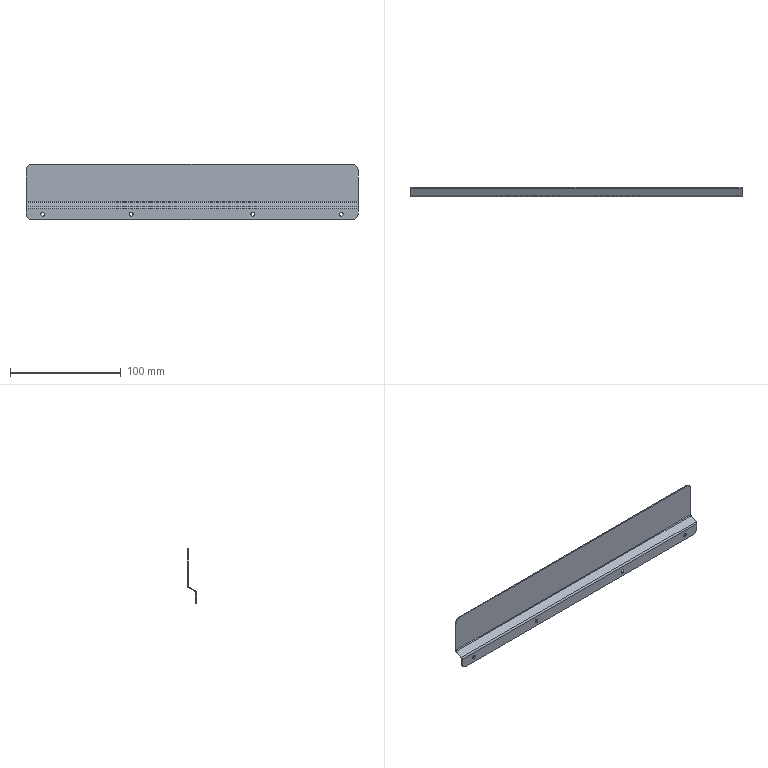Part | SolidWorks | features BaseBody 1 | 1 solid | 26 faces | box 300 x 8.861 x 50.116 mm | volume 16240 mm3 | cylinder 16 | plane 10 | commonest cylinder face diameters 3.5 x8 10 x4 2 x2 4 x2
STEP:
#1=CARTESIAN_POINT('',(-55.,-1.,-1.75));
#2=VERTEX_POINT('',#1);
#3=CARTESIAN_POINT('',(-55.,-1.,1.75));
#4=VERTEX_POINT('',#3);
#5=CARTESIAN_POINT('',(-55.,-1.,0.));
#6=DIRECTION('',(0.,1.,0.));
#7=DIRECTION('',(0.,0.,1.));
#8=AXIS2_PLACEMENT_3D('',#5,#6,#7);
#9=CIRCLE('',#8,1.75);
#10=EDGE_CURVE('',#2,#4,#9,.T.);
#11=ORIENTED_EDGE('',*,*,#10,.F.);
#12=CARTESIAN_POINT('',(-55.,0.,-1.75));
#13=VERTEX_POINT('',#12);
#14=CARTESIAN_POINT('',(-55.,7.861,-1.75));
#15=DIRECTION('',(0.,1.,0.));
#16=VECTOR('',#15,1000.);
#17=LINE('',#14,#16);
#18=EDGE_CURVE('',#2,#13,#17,.T.);
#19=ORIENTED_EDGE('',*,*,#18,.T.);
#20=CARTESIAN_POINT('',(-55.,0.,1.75));
#21=VERTEX_POINT('',#20);
#22=CARTESIAN_POINT('',(-55.,0.,0.));
#23=DIRECTION('',(0.,1.,0.));
#24=DIRECTION('',(0.,0.,1.));
#25=AXIS2_PLACEMENT_3D('',#22,#23,#24);
#26=CIRCLE('',#25,1.75);
#27=EDGE_CURVE('',#13,#21,#26,.T.);
#28=ORIENTED_EDGE('',*,*,#27,.T.);
#29=CARTESIAN_POINT('',(-55.,7.861,1.75));
#30=DIRECTION('',(0.,1.,0.));
#31=VECTOR('',#30,1000.);
#32=LINE('',#29,#31);
#33=EDGE_CURVE('',#4,#21,#32,.T.);
#34=ORIENTED_EDGE('',*,*,#33,.F.);
#35=EDGE_LOOP('',(#11,#19,#28,#34));
#36=FACE_OUTER_BOUND('',#35,.T.);
#37=CARTESIAN_POINT('',(-55.,7.861,0.));
#38=DIRECTION('',(0.,1.,0.));
#39=DIRECTION('',(0.,0.,1.));
#40=AXIS2_PLACEMENT_3D('',#37,#38,#39);
#41=CYLINDRICAL_SURFACE('',#40,1.75);
#42=ADVANCED_FACE('',(#36),#41,.F.);
#43=CARTESIAN_POINT('',(55.,-1.,-1.75));
#44=VERTEX_POINT('',#43);
#45=CARTESIAN_POINT('',(55.,-1.,1.75));
#46=VERTEX_POINT('',#45);
#47=CARTESIAN_POINT('',(55.,-1.,0.));
#48=DIRECTION('',(0.,1.,0.));
#49=DIRECTION('',(0.,0.,1.));
#50=AXIS2_PLACEMENT_3D('',#47,#48,#49);
#51=CIRCLE('',#50,1.75);
#52=EDGE_CURVE('',#44,#46,#51,.T.);
#53=ORIENTED_EDGE('',*,*,#52,.F.);
#54=CARTESIAN_POINT('',(55.,0.,-1.75));
#55=VERTEX_POINT('',#54);
#56=CARTESIAN_POINT('',(55.,7.861,-1.75));
#57=DIRECTION('',(0.,1.,0.));
#58=VECTOR('',#57,1000.);
#59=LINE('',#56,#58);
#60=EDGE_CURVE('',#44,#55,#59,.T.);
#61=ORIENTED_EDGE('',*,*,#60,.T.);
#62=CARTESIAN_POINT('',(55.,0.,1.75));
#63=VERTEX_POINT('',#62);
#64=CARTESIAN_POINT('',(55.,0.,0.));
#65=DIRECTION('',(0.,1.,0.));
#66=DIRECTION('',(0.,0.,1.));
#67=AXIS2_PLACEMENT_3D('',#64,#65,#66);
#68=CIRCLE('',#67,1.75);
#69=EDGE_CURVE('',#55,#63,#68,.T.);
#70=ORIENTED_EDGE('',*,*,#69,.T.);
#71=CARTESIAN_POINT('',(55.,7.861,1.75));
#72=DIRECTION('',(0.,1.,0.));
#73=VECTOR('',#72,1000.);
#74=LINE('',#71,#73);
#75=EDGE_CURVE('',#46,#63,#74,.T.);
#76=ORIENTED_EDGE('',*,*,#75,.F.);
#77=EDGE_LOOP('',(#53,#61,#70,#76));
#78=FACE_OUTER_BOUND('',#77,.T.);
#79=CARTESIAN_POINT('',(55.,7.861,0.));
#80=DIRECTION('',(0.,1.,0.));
#81=DIRECTION('',(0.,0.,1.));
#82=AXIS2_PLACEMENT_3D('',#79,#80,#81);
#83=CYLINDRICAL_SURFACE('',#82,1.75);
#84=ADVANCED_FACE('',(#78),#83,.F.);
#85=CARTESIAN_POINT('',(135.,-1.,-1.75));
#86=VERTEX_POINT('',#85);
#87=CARTESIAN_POINT('',(135.,-1.,1.75));
#88=VERTEX_POINT('',#87);
#89=CARTESIAN_POINT('',(135.,-1.,0.));
#90=DIRECTION('',(0.,1.,0.));
#91=DIRECTION('',(0.,0.,1.));
#92=AXIS2_PLACEMENT_3D('',#89,#90,#91);
#93=CIRCLE('',#92,1.75);
#94=EDGE_CURVE('',#86,#88,#93,.T.);
#95=ORIENTED_EDGE('',*,*,#94,.F.);
#96=CARTESIAN_POINT('',(135.,0.,-1.75));
#97=VERTEX_POINT('',#96);
#98=CARTESIAN_POINT('',(135.,7.861,-1.75));
#99=DIRECTION('',(0.,1.,0.));
#100=VECTOR('',#99,1000.);
#101=LINE('',#98,#100);
#102=EDGE_CURVE('',#86,#97,#101,.T.);
#103=ORIENTED_EDGE('',*,*,#102,.T.);
#104=CARTESIAN_POINT('',(135.,0.,1.75));
#105=VERTEX_POINT('',#104);
#106=CARTESIAN_POINT('',(135.,0.,0.));
#107=DIRECTION('',(0.,1.,0.));
#108=DIRECTION('',(0.,0.,1.));
#109=AXIS2_PLACEMENT_3D('',#106,#107,#108);
#110=CIRCLE('',#109,1.75);
#111=EDGE_CURVE('',#97,#105,#110,.T.);
#112=ORIENTED_EDGE('',*,*,#111,.T.);
#113=CARTESIAN_POINT('',(135.,7.861,1.75));
#114=DIRECTION('',(0.,1.,0.));
#115=VECTOR('',#114,1000.);
#116=LINE('',#113,#115);
#117=EDGE_CURVE('',#88,#105,#116,.T.);
#118=ORIENTED_EDGE('',*,*,#117,.F.);
#119=EDGE_LOOP('',(#95,#103,#112,#118));
#120=FACE_OUTER_BOUND('',#119,.T.);
#121=CARTESIAN_POINT('',(135.,7.861,0.));
#122=DIRECTION('',(0.,1.,0.));
#123=DIRECTION('',(0.,0.,1.));
#124=AXIS2_PLACEMENT_3D('',#121,#122,#123);
#125=CYLINDRICAL_SURFACE('',#124,1.75);
#126=ADVANCED_FACE('',(#120),#125,.F.);
#127=CARTESIAN_POINT('',(-135.,-1.,-1.75));
#128=VERTEX_POINT('',#127);
#129=CARTESIAN_POINT('',(-135.,-1.,1.75));
#130=VERTEX_POINT('',#129);
#131=CARTESIAN_POINT('',(-135.,-1.,0.));
#132=DIRECTION('',(0.,1.,0.));
#133=DIRECTION('',(0.,0.,1.));
#134=AXIS2_PLACEMENT_3D('',#131,#132,#133);
#135=CIRCLE('',#134,1.75);
#136=EDGE_CURVE('',#128,#130,#135,.T.);
#137=ORIENTED_EDGE('',*,*,#136,.F.);
#138=CARTESIAN_POINT('',(-135.,0.,-1.75));
#139=VERTEX_POINT('',#138);
#140=CARTESIAN_POINT('',(-135.,7.861,-1.75));
#141=DIRECTION('',(0.,1.,0.));
#142=VECTOR('',#141,1000.);
#143=LINE('',#140,#142);
#144=EDGE_CURVE('',#128,#139,#143,.T.);
#145=ORIENTED_EDGE('',*,*,#144,.T.);
#146=CARTESIAN_POINT('',(-135.,0.,1.75));
#147=VERTEX_POINT('',#146);
#148=CARTESIAN_POINT('',(-135.,0.,0.));
#149=DIRECTION('',(0.,1.,0.));
#150=DIRECTION('',(0.,0.,1.));
#151=AXIS2_PLACEMENT_3D('',#148,#149,#150);
#152=CIRCLE('',#151,1.75);
#153=EDGE_CURVE('',#139,#147,#152,.T.);
#154=ORIENTED_EDGE('',*,*,#153,.T.);
#155=CARTESIAN_POINT('',(-135.,7.861,1.75));
#156=DIRECTION('',(0.,1.,0.));
#157=VECTOR('',#156,1000.);
#158=LINE('',#155,#157);
#159=EDGE_CURVE('',#130,#147,#158,.T.);
#160=ORIENTED_EDGE('',*,*,#159,.F.);
#161=EDGE_LOOP('',(#137,#145,#154,#160));
#162=FACE_OUTER_BOUND('',#161,.T.);
#163=CARTESIAN_POINT('',(-135.,7.861,0.));
#164=DIRECTION('',(0.,1.,0.));
#165=DIRECTION('',(0.,0.,1.));
#166=AXIS2_PLACEMENT_3D('',#163,#164,#165);
#167=CYLINDRICAL_SURFACE('',#166,1.75);
#168=ADVANCED_FACE('',(#162),#167,.F.);
#169=CARTESIAN_POINT('',(-150.,7.861,40.116));
#170=VERTEX_POINT('',#169);
#171=CARTESIAN_POINT('',(-145.,7.861,45.116));
#172=VERTEX_POINT('',#171);
#173=CARTESIAN_POINT('',(-145.,7.861,40.116));
#174=DIRECTION('',(0.,1.,0.));
#175=DIRECTION('',(0.,0.,-1.));
#176=AXIS2_PLACEMENT_3D('',#173,#174,#175);
#177=CIRCLE('',#176,5.);
#178=EDGE_CURVE('',#170,#172,#177,.T.);
#179=ORIENTED_EDGE('',*,*,#178,.F.);
#180=CARTESIAN_POINT('',(-150.,6.861,40.116));
#181=VERTEX_POINT('',#180);
#182=CARTESIAN_POINT('',(-150.,7.861,40.116));
#183=DIRECTION('',(0.,1.,0.));
#184=VECTOR('',#183,1000.);
#185=LINE('',#182,#184);
#186=EDGE_CURVE('',#181,#170,#185,.T.);
#187=ORIENTED_EDGE('',*,*,#186,.F.);
#188=CARTESIAN_POINT('',(-145.,6.861,45.116));
#189=VERTEX_POINT('',#188);
#190=CARTESIAN_POINT('',(-145.,6.861,40.116));
#191=DIRECTION('',(0.,-1.,0.));
#192=DIRECTION('',(0.,0.,-1.));
#193=AXIS2_PLACEMENT_3D('',#190,#191,#192);
#194=CIRCLE('',#193,5.);
#195=EDGE_CURVE('',#189,#181,#194,.T.);
#196=ORIENTED_EDGE('',*,*,#195,.F.);
#197=CARTESIAN_POINT('',(-145.,7.861,45.116));
#198=DIRECTION('',(0.,-1.,0.));
#199=VECTOR('',#198,1000.);
#200=LINE('',#197,#199);
#201=EDGE_CURVE('',#172,#189,#200,.T.);
#202=ORIENTED_EDGE('',*,*,#201,.F.);
#203=EDGE_LOOP('',(#179,#187,#196,#202));
#204=FACE_OUTER_BOUND('',#203,.T.);
#205=CARTESIAN_POINT('',(-145.,7.861,40.116));
#206=DIRECTION('',(0.,-1.,0.));
#207=DIRECTION('',(0.,0.,-1.));
#208=AXIS2_PLACEMENT_3D('',#205,#206,#207);
#209=CYLINDRICAL_SURFACE('',#208,5.);
#210=ADVANCED_FACE('',(#204),#209,.T.);
#211=CARTESIAN_POINT('',(145.,7.861,45.116));
#212=VERTEX_POINT('',#211);
#213=CARTESIAN_POINT('',(150.,7.861,40.116));
#214=VERTEX_POINT('',#213);
#215=CARTESIAN_POINT('',(145.,7.861,40.116));
#216=DIRECTION('',(0.,1.,0.));
#217=DIRECTION('',(0.,0.,-1.));
#218=AXIS2_PLACEMENT_3D('',#215,#216,#217);
#219=CIRCLE('',#218,5.);
#220=EDGE_CURVE('',#212,#214,#219,.T.);
#221=ORIENTED_EDGE('',*,*,#220,.F.);
#222=CARTESIAN_POINT('',(145.,6.861,45.116));
#223=VERTEX_POINT('',#222);
#224=CARTESIAN_POINT('',(145.,7.861,45.116));
#225=DIRECTION('',(0.,1.,0.));
#226=VECTOR('',#225,1000.);
#227=LINE('',#224,#226);
#228=EDGE_CURVE('',#223,#212,#227,.T.);
#229=ORIENTED_EDGE('',*,*,#228,.F.);
#230=CARTESIAN_POINT('',(150.,6.861,40.116));
#231=VERTEX_POINT('',#230);
#232=CARTESIAN_POINT('',(145.,6.861,40.116));
#233=DIRECTION('',(0.,-1.,0.));
#234=DIRECTION('',(0.,0.,-1.));
#235=AXIS2_PLACEMENT_3D('',#232,#233,#234);
#236=CIRCLE('',#235,5.);
#237=EDGE_CURVE('',#231,#223,#236,.T.);
#238=ORIENTED_EDGE('',*,*,#237,.F.);
#239=CARTESIAN_POINT('',(150.,7.861,40.116));
#240=DIRECTION('',(0.,-1.,0.));
#241=VECTOR('',#240,1000.);
#242=LINE('',#239,#241);
#243=EDGE_CURVE('',#214,#231,#242,.T.);
#244=ORIENTED_EDGE('',*,*,#243,.F.);
#245=EDGE_LOOP('',(#221,#229,#238,#244));
#246=FACE_OUTER_BOUND('',#245,.T.);
#247=CARTESIAN_POINT('',(145.,7.861,40.116));
#248=DIRECTION('',(0.,-1.,0.));
#249=DIRECTION('',(0.,0.,-1.));
#250=AXIS2_PLACEMENT_3D('',#247,#248,#249);
#251=CYLINDRICAL_SURFACE('',#250,5.);
#252=ADVANCED_FACE('',(#246),#251,.T.);
#253=CARTESIAN_POINT('',(-150.,-1.,0.));
#254=VERTEX_POINT('',#253);
#255=CARTESIAN_POINT('',(-145.,-1.,-5.));
#256=VERTEX_POINT('',#255);
#257=CARTESIAN_POINT('',(-145.,-1.,0.));
#258=DIRECTION('',(0.,-1.,0.));
#259=DIRECTION('',(0.,0.,1.));
#260=AXIS2_PLACEMENT_3D('',#257,#258,#259);
#261=CIRCLE('',#260,5.);
#262=EDGE_CURVE('',#254,#256,#261,.T.);
#263=ORIENTED_EDGE('',*,*,#262,.F.);
#264=CARTESIAN_POINT('',(-150.,0.,0.));
#265=VERTEX_POINT('',#264);
#266=CARTESIAN_POINT('',(-150.,-1.,0.));
#267=DIRECTION('',(0.,-1.,0.));
#268=VECTOR('',#267,1000.);
#269=LINE('',#266,#268);
#270=EDGE_CURVE('',#265,#254,#269,.T.);
#271=ORIENTED_EDGE('',*,*,#270,.F.);
#272=CARTESIAN_POINT('',(-145.,0.,-5.));
#273=VERTEX_POINT('',#272);
#274=CARTESIAN_POINT('',(-145.,0.,0.));
#275=DIRECTION('',(0.,1.,0.));
#276=DIRECTION('',(0.,0.,1.));
#277=AXIS2_PLACEMENT_3D('',#274,#275,#276);
#278=CIRCLE('',#277,5.);
#279=EDGE_CURVE('',#273,#265,#278,.T.);
#280=ORIENTED_EDGE('',*,*,#279,.F.);
#281=CARTESIAN_POINT('',(-145.,-1.,-5.));
#282=DIRECTION('',(0.,1.,0.));
#283=VECTOR('',#282,1000.);
#284=LINE('',#281,#283);
#285=EDGE_CURVE('',#256,#273,#284,.T.);
#286=ORIENTED_EDGE('',*,*,#285,.F.);
#287=EDGE_LOOP('',(#263,#271,#280,#286));
#288=FACE_OUTER_BOUND('',#287,.T.);
#289=CARTESIAN_POINT('',(-145.,-1.,0.));
#290=DIRECTION('',(0.,1.,0.));
#291=DIRECTION('',(0.,0.,1.));
#292=AXIS2_PLACEMENT_3D('',#289,#290,#291);
#293=CYLINDRICAL_SURFACE('',#292,5.);
#294=ADVANCED_FACE('',(#288),#293,.T.);
#295=CARTESIAN_POINT('',(145.,-1.,-5.));
#296=VERTEX_POINT('',#295);
#297=CARTESIAN_POINT('',(150.,-1.,0.));
#298=VERTEX_POINT('',#297);
#299=CARTESIAN_POINT('',(145.,-1.,0.));
#300=DIRECTION('',(0.,-1.,0.));
#301=DIRECTION('',(0.,0.,1.));
#302=AXIS2_PLACEMENT_3D('',#299,#300,#301);
#303=CIRCLE('',#302,5.);
#304=EDGE_CURVE('',#296,#298,#303,.T.);
#305=ORIENTED_EDGE('',*,*,#304,.F.);
#306=CARTESIAN_POINT('',(145.,0.,-5.));
#307=VERTEX_POINT('',#306);
#308=CARTESIAN_POINT('',(145.,-1.,-5.));
#309=DIRECTION('',(0.,-1.,0.));
#310=VECTOR('',#309,1000.);
#311=LINE('',#308,#310);
#312=EDGE_CURVE('',#307,#296,#311,.T.);
#313=ORIENTED_EDGE('',*,*,#312,.F.);
#314=CARTESIAN_POINT('',(150.,0.,0.));
#315=VERTEX_POINT('',#314);
#316=CARTESIAN_POINT('',(145.,0.,0.));
#317=DIRECTION('',(0.,1.,0.));
#318=DIRECTION('',(0.,0.,1.));
#319=AXIS2_PLACEMENT_3D('',#316,#317,#318);
#320=CIRCLE('',#319,5.);
#321=EDGE_CURVE('',#315,#307,#320,.T.);
#322=ORIENTED_EDGE('',*,*,#321,.F.);
#323=CARTESIAN_POINT('',(150.,-1.,0.));
#324=DIRECTION('',(0.,1.,0.));
#325=VECTOR('',#324,1000.);
#326=LINE('',#323,#325);
#327=EDGE_CURVE('',#298,#315,#326,.T.);
#328=ORIENTED_EDGE('',*,*,#327,.F.);
#329=EDGE_LOOP('',(#305,#313,#322,#328));
#330=FACE_OUTER_BOUND('',#329,.T.);
#331=CARTESIAN_POINT('',(145.,-1.,0.));
#332=DIRECTION('',(0.,1.,0.));
#333=DIRECTION('',(0.,0.,1.));
#334=AXIS2_PLACEMENT_3D('',#331,#332,#333);
#335=CYLINDRICAL_SURFACE('',#334,5.);
#336=ADVANCED_FACE('',(#330),#335,.T.);
#337=CARTESIAN_POINT('',(150.,6.861,45.116));
#338=DIRECTION('',(1.,0.,0.));
#339=VECTOR('',#338,1000.);
#340=LINE('',#337,#339);
#341=EDGE_CURVE('',#189,#223,#340,.T.);
#342=ORIENTED_EDGE('',*,*,#341,.T.);
#343=ORIENTED_EDGE('',*,*,#228,.T.);
#344=CARTESIAN_POINT('',(0.,7.861,45.116));
#345=DIRECTION('',(1.,0.,0.));
#346=VECTOR('',#345,1000.);
#347=LINE('',#344,#346);
#348=EDGE_CURVE('',#172,#212,#347,.T.);
#349=ORIENTED_EDGE('',*,*,#348,.F.);
#350=ORIENTED_EDGE('',*,*,#201,.T.);
#351=EDGE_LOOP('',(#342,#343,#349,#350));
#352=FACE_OUTER_BOUND('',#351,.T.);
#353=CARTESIAN_POINT('',(150.,7.861,45.116));
#354=DIRECTION('',(0.,0.,-1.));
#355=DIRECTION('',(-1.,0.,0.));
#356=AXIS2_PLACEMENT_3D('',#353,#354,#355);
#357=PLANE('',#356);
#358=ADVANCED_FACE('',(#352),#357,.F.);
#359=CARTESIAN_POINT('',(150.,6.861,11.271));
#360=VERTEX_POINT('',#359);
#361=CARTESIAN_POINT('',(150.,6.861,10.693));
#362=DIRECTION('',(0.,0.,-1.));
#363=VECTOR('',#362,1000.);
#364=LINE('',#361,#363);
#365=EDGE_CURVE('',#231,#360,#364,.T.);
#366=ORIENTED_EDGE('',*,*,#365,.F.);
#367=ORIENTED_EDGE('',*,*,#237,.T.);
#368=ORIENTED_EDGE('',*,*,#341,.F.);
#369=ORIENTED_EDGE('',*,*,#195,.T.);
#370=CARTESIAN_POINT('',(-150.,6.861,11.271));
#371=VERTEX_POINT('',#370);
#372=CARTESIAN_POINT('',(-150.,6.861,45.116));
#373=DIRECTION('',(0.,0.,1.));
#374=VECTOR('',#373,1000.);
#375=LINE('',#372,#374);
#376=EDGE_CURVE('',#371,#181,#375,.T.);
#377=ORIENTED_EDGE('',*,*,#376,.F.);
#378=CARTESIAN_POINT('',(150.,6.861,11.271));
#379=DIRECTION('',(-1.,0.,0.));
#380=VECTOR('',#379,1000.);
#381=LINE('',#378,#380);
#382=EDGE_CURVE('',#360,#371,#381,.T.);
#383=ORIENTED_EDGE('',*,*,#382,.F.);
#384=EDGE_LOOP('',(#366,#367,#368,#369,#377,#383));
#385=FACE_OUTER_BOUND('',#384,.T.);
#386=CARTESIAN_POINT('',(0.,6.861,0.2887));
#387=DIRECTION('',(0.,-1.,0.));
#388=DIRECTION('',(0.,0.,-1.));
#389=AXIS2_PLACEMENT_3D('',#386,#387,#388);
#390=PLANE('',#389);
#391=ADVANCED_FACE('',(#385),#390,.T.);
#392=ORIENTED_EDGE('',*,*,#348,.T.);
#393=ORIENTED_EDGE('',*,*,#220,.T.);
#394=CARTESIAN_POINT('',(150.,7.861,11.271));
#395=VERTEX_POINT('',#394);
#396=CARTESIAN_POINT('',(150.,7.861,0.2887));
#397=DIRECTION('',(0.,0.,-1.));
#398=VECTOR('',#397,1000.);
#399=LINE('',#396,#398);
#400=EDGE_CURVE('',#214,#395,#399,.T.);
#401=ORIENTED_EDGE('',*,*,#400,.T.);
#402=CARTESIAN_POINT('',(-150.,7.861,11.271));
#403=VERTEX_POINT('',#402);
#404=CARTESIAN_POINT('',(150.,7.861,11.271));
#405=DIRECTION('',(1.,0.,0.));
#406=VECTOR('',#405,1000.);
#407=LINE('',#404,#406);
#408=EDGE_CURVE('',#403,#395,#407,.T.);
#409=ORIENTED_EDGE('',*,*,#408,.F.);
#410=CARTESIAN_POINT('',(-150.,7.861,0.2887));
#411=DIRECTION('',(0.,0.,1.));
#412=VECTOR('',#411,1000.);
#413=LINE('',#410,#412);
#414=EDGE_CURVE('',#403,#170,#413,.T.);
#415=ORIENTED_EDGE('',*,*,#414,.T.);
#416=ORIENTED_EDGE('',*,*,#178,.T.);
#417=EDGE_LOOP('',(#392,#393,#401,#409,#415,#416));
#418=FACE_OUTER_BOUND('',#417,.T.);
#419=CARTESIAN_POINT('',(0.,7.861,0.2887));
#420=DIRECTION('',(0.,-1.,0.));
#421=DIRECTION('',(0.,0.,-1.));
#422=AXIS2_PLACEMENT_3D('',#419,#420,#421);
#423=PLANE('',#422);
#424=ADVANCED_FACE('',(#418),#423,.F.);
#425=CARTESIAN_POINT('',(150.,6.361,10.405));
#426=VERTEX_POINT('',#425);
#427=CARTESIAN_POINT('',(-150.,6.361,10.405));
#428=VERTEX_POINT('',#427);
#429=CARTESIAN_POINT('',(0.,6.361,10.405));
#430=DIRECTION('',(-1.,0.,0.));
#431=VECTOR('',#430,1000.);
#432=LINE('',#429,#431);
#433=EDGE_CURVE('',#426,#428,#432,.T.);
#434=ORIENTED_EDGE('',*,*,#433,.F.);
#435=CARTESIAN_POINT('',(150.,5.861,11.271));
#436=DIRECTION('',(1.,0.,0.));
#437=DIRECTION('',(0.,0.,1.));
#438=AXIS2_PLACEMENT_3D('',#435,#436,#437);
#439=CIRCLE('',#438,1.);
#440=EDGE_CURVE('',#426,#360,#439,.T.);
#441=ORIENTED_EDGE('',*,*,#440,.T.);
#442=ORIENTED_EDGE('',*,*,#382,.T.);
#443=CARTESIAN_POINT('',(-150.,5.861,11.271));
#444=DIRECTION('',(-1.,0.,0.));
#445=DIRECTION('',(0.,0.,1.));
#446=AXIS2_PLACEMENT_3D('',#443,#444,#445);
#447=CIRCLE('',#446,1.);
#448=EDGE_CURVE('',#371,#428,#447,.T.);
#449=ORIENTED_EDGE('',*,*,#448,.T.);
#450=EDGE_LOOP('',(#434,#441,#442,#449));
#451=FACE_OUTER_BOUND('',#450,.T.);
#452=CARTESIAN_POINT('',(-150.,5.861,11.271));
#453=DIRECTION('',(-1.,0.,0.));
#454=DIRECTION('',(0.,1.,0.));
#455=AXIS2_PLACEMENT_3D('',#452,#453,#454);
#456=CYLINDRICAL_SURFACE('',#455,1.);
#457=ADVANCED_FACE('',(#451),#456,.F.);
#458=CARTESIAN_POINT('',(150.,6.861,9.539));
#459=VERTEX_POINT('',#458);
#460=CARTESIAN_POINT('',(-150.,6.861,9.539));
#461=VERTEX_POINT('',#460);
#462=CARTESIAN_POINT('',(-150.,6.861,9.539));
#463=DIRECTION('',(-1.,0.,0.));
#464=VECTOR('',#463,1000.);
#465=LINE('',#462,#464);
#466=EDGE_CURVE('',#459,#461,#465,.T.);
#467=ORIENTED_EDGE('',*,*,#466,.T.);
#468=CARTESIAN_POINT('',(-150.,5.861,11.271));
#469=DIRECTION('',(-1.,0.,0.));
#470=DIRECTION('',(0.,0.,1.));
#471=AXIS2_PLACEMENT_3D('',#468,#469,#470);
#472=CIRCLE('',#471,2.);
#473=EDGE_CURVE('',#403,#461,#472,.T.);
#474=ORIENTED_EDGE('',*,*,#473,.F.);
#475=ORIENTED_EDGE('',*,*,#408,.T.);
#476=CARTESIAN_POINT('',(150.,5.861,11.271));
#477=DIRECTION('',(1.,0.,0.));
#478=DIRECTION('',(0.,0.,1.));
#479=AXIS2_PLACEMENT_3D('',#476,#477,#478);
#480=CIRCLE('',#479,2.);
#481=EDGE_CURVE('',#459,#395,#480,.T.);
#482=ORIENTED_EDGE('',*,*,#481,.F.);
#483=EDGE_LOOP('',(#467,#474,#475,#482));
#484=FACE_OUTER_BOUND('',#483,.T.);
#485=CARTESIAN_POINT('',(-150.,5.861,11.271));
#486=DIRECTION('',(-1.,0.,0.));
#487=DIRECTION('',(0.,1.,0.));
#488=AXIS2_PLACEMENT_3D('',#485,#486,#487);
#489=CYLINDRICAL_SURFACE('',#488,2.);
#490=ADVANCED_FACE('',(#484),#489,.T.);
#491=CARTESIAN_POINT('',(150.,0.5,5.866));
#492=VERTEX_POINT('',#491);
#493=CARTESIAN_POINT('',(150.,6.861,9.539));
#494=DIRECTION('',(0.,0.866,0.5));
#495=VECTOR('',#494,1000.);
#496=LINE('',#493,#495);
#497=EDGE_CURVE('',#492,#459,#496,.T.);
#498=ORIENTED_EDGE('',*,*,#497,.F.);
#499=CARTESIAN_POINT('',(-150.,0.5,5.866));
#500=VERTEX_POINT('',#499);
#501=CARTESIAN_POINT('',(-150.,0.5,5.866));
#502=DIRECTION('',(1.,0.,0.));
#503=VECTOR('',#502,1000.);
#504=LINE('',#501,#503);
#505=EDGE_CURVE('',#500,#492,#504,.T.);
#506=ORIENTED_EDGE('',*,*,#505,.F.);
#507=CARTESIAN_POINT('',(-150.,0.,5.577));
#508=DIRECTION('',(0.,-0.866,-0.5));
#509=VECTOR('',#508,1000.);
#510=LINE('',#507,#509);
#511=EDGE_CURVE('',#461,#500,#510,.T.);
#512=ORIENTED_EDGE('',*,*,#511,.F.);
#513=ORIENTED_EDGE('',*,*,#466,.F.);
#514=EDGE_LOOP('',(#498,#506,#512,#513));
#515=FACE_OUTER_BOUND('',#514,.T.);
#516=CARTESIAN_POINT('',(0.,-2.165,4.327));
#517=DIRECTION('',(0.,0.5,-0.866));
#518=DIRECTION('',(-1.,0.,0.));
#519=AXIS2_PLACEMENT_3D('',#516,#517,#518);
#520=PLANE('',#519);
#521=ADVANCED_FACE('',(#515),#520,.T.);
#522=CARTESIAN_POINT('',(150.,0.,6.732));
#523=VERTEX_POINT('',#522);
#524=CARTESIAN_POINT('',(-150.,0.,6.732));
#525=VERTEX_POINT('',#524);
#526=CARTESIAN_POINT('',(-150.,0.,6.732));
#527=DIRECTION('',(-1.,0.,0.));
#528=VECTOR('',#527,1000.);
#529=LINE('',#526,#528);
#530=EDGE_CURVE('',#523,#525,#529,.T.);
#531=ORIENTED_EDGE('',*,*,#530,.F.);
#532=CARTESIAN_POINT('',(150.,-2.665,5.193));
#533=DIRECTION('',(0.,0.866,0.5));
#534=VECTOR('',#533,1000.);
#535=LINE('',#532,#534);
#536=EDGE_CURVE('',#523,#426,#535,.T.);
#537=ORIENTED_EDGE('',*,*,#536,.T.);
#538=ORIENTED_EDGE('',*,*,#433,.T.);
#539=CARTESIAN_POINT('',(-150.,-2.665,5.193));
#540=DIRECTION('',(0.,-0.866,-0.5));
#541=VECTOR('',#540,1000.);
#542=LINE('',#539,#541);
#543=EDGE_CURVE('',#428,#525,#542,.T.);
#544=ORIENTED_EDGE('',*,*,#543,.T.);
#545=EDGE_LOOP('',(#531,#537,#538,#544));
#546=FACE_OUTER_BOUND('',#545,.T.);
#547=CARTESIAN_POINT('',(0.,-2.665,5.193));
#548=DIRECTION('',(0.,0.5,-0.866));
#549=DIRECTION('',(-1.,0.,0.));
#550=AXIS2_PLACEMENT_3D('',#547,#548,#549);
#551=PLANE('',#550);
#552=ADVANCED_FACE('',(#546),#551,.F.);
#553=CARTESIAN_POINT('',(-150.,0.,5.));
#554=VERTEX_POINT('',#553);
#555=CARTESIAN_POINT('',(150.,0.,5.));
#556=VERTEX_POINT('',#555);
#557=CARTESIAN_POINT('',(-150.,0.,5.));
#558=DIRECTION('',(1.,0.,0.));
#559=VECTOR('',#558,1000.);
#560=LINE('',#557,#559);
#561=EDGE_CURVE('',#554,#556,#560,.T.);
#562=ORIENTED_EDGE('',*,*,#561,.F.);
#563=CARTESIAN_POINT('',(-150.,1.,5.));
#564=DIRECTION('',(-1.,0.,0.));
#565=DIRECTION('',(0.,0.,-1.));
#566=AXIS2_PLACEMENT_3D('',#563,#564,#565);
#567=CIRCLE('',#566,1.);
#568=EDGE_CURVE('',#554,#500,#567,.T.);
#569=ORIENTED_EDGE('',*,*,#568,.T.);
#570=ORIENTED_EDGE('',*,*,#505,.T.);
#571=CARTESIAN_POINT('',(150.,1.,5.));
#572=DIRECTION('',(1.,0.,0.));
#573=DIRECTION('',(0.,0.,-1.));
#574=AXIS2_PLACEMENT_3D('',#571,#572,#573);
#575=CIRCLE('',#574,1.);
#576=EDGE_CURVE('',#492,#556,#575,.T.);
#577=ORIENTED_EDGE('',*,*,#576,.T.);
#578=EDGE_LOOP('',(#562,#569,#570,#577));
#579=FACE_OUTER_BOUND('',#578,.T.);
#580=CARTESIAN_POINT('',(150.,1.,5.));
#581=DIRECTION('',(1.,0.,0.));
#582=DIRECTION('',(0.,-0.5,0.866));
#583=AXIS2_PLACEMENT_3D('',#580,#581,#582);
#584=CYLINDRICAL_SURFACE('',#583,1.);
#585=ADVANCED_FACE('',(#579),#584,.F.);
#586=CARTESIAN_POINT('',(-150.,-1.,5.));
#587=VERTEX_POINT('',#586);
#588=CARTESIAN_POINT('',(150.,-1.,5.));
#589=VERTEX_POINT('',#588);
#590=CARTESIAN_POINT('',(-150.,-1.,5.));
#591=DIRECTION('',(1.,0.,0.));
#592=VECTOR('',#591,1000.);
#593=LINE('',#590,#592);
#594=EDGE_CURVE('',#587,#589,#593,.T.);
#595=ORIENTED_EDGE('',*,*,#594,.T.);
#596=CARTESIAN_POINT('',(150.,1.,5.));
#597=DIRECTION('',(1.,0.,0.));
#598=DIRECTION('',(0.,0.,-1.));
#599=AXIS2_PLACEMENT_3D('',#596,#597,#598);
#600=CIRCLE('',#599,2.);
#601=EDGE_CURVE('',#523,#589,#600,.T.);
#602=ORIENTED_EDGE('',*,*,#601,.F.);
#603=ORIENTED_EDGE('',*,*,#530,.T.);
#604=CARTESIAN_POINT('',(-150.,1.,5.));
#605=DIRECTION('',(-1.,0.,0.));
#606=DIRECTION('',(0.,0.,-1.));
#607=AXIS2_PLACEMENT_3D('',#604,#605,#606);
#608=CIRCLE('',#607,2.);
#609=EDGE_CURVE('',#587,#525,#608,.T.);
#610=ORIENTED_EDGE('',*,*,#609,.F.);
#611=EDGE_LOOP('',(#595,#602,#603,#610));
#612=FACE_OUTER_BOUND('',#611,.T.);
#613=CARTESIAN_POINT('',(150.,1.,5.));
#614=DIRECTION('',(1.,0.,0.));
#615=DIRECTION('',(0.,-0.5,0.866));
#616=AXIS2_PLACEMENT_3D('',#613,#614,#615);
#617=CYLINDRICAL_SURFACE('',#616,2.);
#618=ADVANCED_FACE('',(#612),#617,.T.);
#619=CARTESIAN_POINT('',(-135.,0.,0.));
#620=DIRECTION('',(0.,1.,0.));
#621=DIRECTION('',(0.,0.,1.));
#622=AXIS2_PLACEMENT_3D('',#619,#620,#621);
#623=CIRCLE('',#622,1.75);
#624=EDGE_CURVE('',#147,#139,#623,.T.);
#625=ORIENTED_EDGE('',*,*,#624,.F.);
#626=ORIENTED_EDGE('',*,*,#153,.F.);
#627=EDGE_LOOP('',(#625,#626));
#628=FACE_BOUND('',#627,.T.);
#629=CARTESIAN_POINT('',(135.,0.,0.));
#630=DIRECTION('',(0.,1.,0.));
#631=DIRECTION('',(0.,0.,1.));
#632=AXIS2_PLACEMENT_3D('',#629,#630,#631);
#633=CIRCLE('',#632,1.75);
#634=EDGE_CURVE('',#105,#97,#633,.T.);
#635=ORIENTED_EDGE('',*,*,#634,.F.);
#636=ORIENTED_EDGE('',*,*,#111,.F.);
#637=EDGE_LOOP('',(#635,#636));
#638=FACE_BOUND('',#637,.T.);
#639=CARTESIAN_POINT('',(55.,0.,0.));
#640=DIRECTION('',(0.,1.,0.));
#641=DIRECTION('',(0.,0.,1.));
#642=AXIS2_PLACEMENT_3D('',#639,#640,#641);
#643=CIRCLE('',#642,1.75);
#644=EDGE_CURVE('',#63,#55,#643,.T.);
#645=ORIENTED_EDGE('',*,*,#644,.F.);
#646=ORIENTED_EDGE('',*,*,#69,.F.);
#647=EDGE_LOOP('',(#645,#646));
#648=FACE_BOUND('',#647,.T.);
#649=CARTESIAN_POINT('',(-55.,0.,0.));
#650=DIRECTION('',(0.,1.,0.));
#651=DIRECTION('',(0.,0.,1.));
#652=AXIS2_PLACEMENT_3D('',#649,#650,#651);
#653=CIRCLE('',#652,1.75);
#654=EDGE_CURVE('',#21,#13,#653,.T.);
#655=ORIENTED_EDGE('',*,*,#654,.F.);
#656=ORIENTED_EDGE('',*,*,#27,.F.);
#657=EDGE_LOOP('',(#655,#656));
#658=FACE_BOUND('',#657,.T.);
#659=CARTESIAN_POINT('',(150.,0.,-5.));
#660=DIRECTION('',(0.,0.,-1.));
#661=VECTOR('',#660,1000.);
#662=LINE('',#659,#661);
#663=EDGE_CURVE('',#556,#315,#662,.T.);
#664=ORIENTED_EDGE('',*,*,#663,.T.);
#665=ORIENTED_EDGE('',*,*,#321,.T.);
#666=CARTESIAN_POINT('',(-150.,0.,-5.));
#667=DIRECTION('',(-1.,0.,0.));
#668=VECTOR('',#667,1000.);
#669=LINE('',#666,#668);
#670=EDGE_CURVE('',#307,#273,#669,.T.);
#671=ORIENTED_EDGE('',*,*,#670,.T.);
#672=ORIENTED_EDGE('',*,*,#279,.T.);
#673=CARTESIAN_POINT('',(-150.,0.,-5.));
#674=DIRECTION('',(0.,0.,1.));
#675=VECTOR('',#674,1000.);
#676=LINE('',#673,#675);
#677=EDGE_CURVE('',#265,#554,#676,.T.);
#678=ORIENTED_EDGE('',*,*,#677,.T.);
#679=ORIENTED_EDGE('',*,*,#561,.T.);
#680=EDGE_LOOP('',(#664,#665,#671,#672,#678,#679));
#681=FACE_OUTER_BOUND('',#680,.T.);
#682=CARTESIAN_POINT('',(0.,0.,0.));
#683=DIRECTION('',(0.,1.,0.));
#684=DIRECTION('',(1.,0.,0.));
#685=AXIS2_PLACEMENT_3D('',#682,#683,#684);
#686=PLANE('',#685);
#687=ADVANCED_FACE('',(#628,#638,#648,#658,#681),#686,.T.);
#688=CARTESIAN_POINT('',(-135.,-1.,0.));
#689=DIRECTION('',(0.,1.,0.));
#690=DIRECTION('',(0.,0.,1.));
#691=AXIS2_PLACEMENT_3D('',#688,#689,#690);
#692=CIRCLE('',#691,1.75);
#693=EDGE_CURVE('',#130,#128,#692,.T.);
#694=ORIENTED_EDGE('',*,*,#693,.T.);
#695=ORIENTED_EDGE('',*,*,#136,.T.);
#696=EDGE_LOOP('',(#694,#695));
#697=FACE_BOUND('',#696,.T.);
#698=CARTESIAN_POINT('',(135.,-1.,0.));
#699=DIRECTION('',(0.,1.,0.));
#700=DIRECTION('',(0.,0.,1.));
#701=AXIS2_PLACEMENT_3D('',#698,#699,#700);
#702=CIRCLE('',#701,1.75);
#703=EDGE_CURVE('',#88,#86,#702,.T.);
#704=ORIENTED_EDGE('',*,*,#703,.T.);
#705=ORIENTED_EDGE('',*,*,#94,.T.);
#706=EDGE_LOOP('',(#704,#705));
#707=FACE_BOUND('',#706,.T.);
#708=CARTESIAN_POINT('',(55.,-1.,0.));
#709=DIRECTION('',(0.,1.,0.));
#710=DIRECTION('',(0.,0.,1.));
#711=AXIS2_PLACEMENT_3D('',#708,#709,#710);
#712=CIRCLE('',#711,1.75);
#713=EDGE_CURVE('',#46,#44,#712,.T.);
#714=ORIENTED_EDGE('',*,*,#713,.T.);
#715=ORIENTED_EDGE('',*,*,#52,.T.);
#716=EDGE_LOOP('',(#714,#715));
#717=FACE_BOUND('',#716,.T.);
#718=CARTESIAN_POINT('',(-55.,-1.,0.));
#719=DIRECTION('',(0.,1.,0.));
#720=DIRECTION('',(0.,0.,1.));
#721=AXIS2_PLACEMENT_3D('',#718,#719,#720);
#722=CIRCLE('',#721,1.75);
#723=EDGE_CURVE('',#4,#2,#722,.T.);
#724=ORIENTED_EDGE('',*,*,#723,.T.);
#725=ORIENTED_EDGE('',*,*,#10,.T.);
#726=EDGE_LOOP('',(#724,#725));
#727=FACE_BOUND('',#726,.T.);
#728=CARTESIAN_POINT('',(-150.,-1.,-5.));
#729=DIRECTION('',(-1.,0.,0.));
#730=VECTOR('',#729,1000.);
#731=LINE('',#728,#730);
#732=EDGE_CURVE('',#296,#256,#731,.T.);
#733=ORIENTED_EDGE('',*,*,#732,.F.);
#734=ORIENTED_EDGE('',*,*,#304,.T.);
#735=CARTESIAN_POINT('',(150.,-1.,-5.));
#736=DIRECTION('',(0.,0.,-1.));
#737=VECTOR('',#736,1000.);
#738=LINE('',#735,#737);
#739=EDGE_CURVE('',#589,#298,#738,.T.);
#740=ORIENTED_EDGE('',*,*,#739,.F.);
#741=ORIENTED_EDGE('',*,*,#594,.F.);
#742=CARTESIAN_POINT('',(-150.,-1.,-5.));
#743=DIRECTION('',(0.,0.,1.));
#744=VECTOR('',#743,1000.);
#745=LINE('',#742,#744);
#746=EDGE_CURVE('',#254,#587,#745,.T.);
#747=ORIENTED_EDGE('',*,*,#746,.F.);
#748=ORIENTED_EDGE('',*,*,#262,.T.);
#749=EDGE_LOOP('',(#733,#734,#740,#741,#747,#748));
#750=FACE_OUTER_BOUND('',#749,.T.);
#751=CARTESIAN_POINT('',(0.,-1.,0.));
#752=DIRECTION('',(0.,1.,0.));
#753=DIRECTION('',(1.,0.,0.));
#754=AXIS2_PLACEMENT_3D('',#751,#752,#753);
#755=PLANE('',#754);
#756=ADVANCED_FACE('',(#697,#707,#717,#727,#750),#755,.F.);
#757=ORIENTED_EDGE('',*,*,#670,.F.);
#758=ORIENTED_EDGE('',*,*,#312,.T.);
#759=ORIENTED_EDGE('',*,*,#732,.T.);
#760=ORIENTED_EDGE('',*,*,#285,.T.);
#761=EDGE_LOOP('',(#757,#758,#759,#760));
#762=FACE_OUTER_BOUND('',#761,.T.);
#763=CARTESIAN_POINT('',(-150.,-1.,-5.));
#764=DIRECTION('',(0.,0.,-1.));
#765=DIRECTION('',(0.,-1.,0.));
#766=AXIS2_PLACEMENT_3D('',#763,#764,#765);
#767=PLANE('',#766);
#768=ADVANCED_FACE('',(#762),#767,.T.);
#769=ORIENTED_EDGE('',*,*,#677,.F.);
#770=ORIENTED_EDGE('',*,*,#270,.T.);
#771=ORIENTED_EDGE('',*,*,#746,.T.);
#772=ORIENTED_EDGE('',*,*,#609,.T.);
#773=ORIENTED_EDGE('',*,*,#543,.F.);
#774=ORIENTED_EDGE('',*,*,#448,.F.);
#775=ORIENTED_EDGE('',*,*,#376,.T.);
#776=ORIENTED_EDGE('',*,*,#186,.T.);
#777=ORIENTED_EDGE('',*,*,#414,.F.);
#778=ORIENTED_EDGE('',*,*,#473,.T.);
#779=ORIENTED_EDGE('',*,*,#511,.T.);
#780=ORIENTED_EDGE('',*,*,#568,.F.);
#781=EDGE_LOOP('',(#769,#770,#771,#772,#773,#774,#775,#776,#777,#778,#779,#780));
#782=FACE_OUTER_BOUND('',#781,.T.);
#783=CARTESIAN_POINT('',(-150.,-1.,-5.));
#784=DIRECTION('',(-1.,0.,0.));
#785=DIRECTION('',(0.,0.,1.));
#786=AXIS2_PLACEMENT_3D('',#783,#784,#785);
#787=PLANE('',#786);
#788=ADVANCED_FACE('',(#782),#787,.T.);
#789=ORIENTED_EDGE('',*,*,#739,.T.);
#790=ORIENTED_EDGE('',*,*,#327,.T.);
#791=ORIENTED_EDGE('',*,*,#663,.F.);
#792=ORIENTED_EDGE('',*,*,#576,.F.);
#793=ORIENTED_EDGE('',*,*,#497,.T.);
#794=ORIENTED_EDGE('',*,*,#481,.T.);
#795=ORIENTED_EDGE('',*,*,#400,.F.);
#796=ORIENTED_EDGE('',*,*,#243,.T.);
#797=ORIENTED_EDGE('',*,*,#365,.T.);
#798=ORIENTED_EDGE('',*,*,#440,.F.);
#799=ORIENTED_EDGE('',*,*,#536,.F.);
#800=ORIENTED_EDGE('',*,*,#601,.T.);
#801=EDGE_LOOP('',(#789,#790,#791,#792,#793,#794,#795,#796,#797,#798,#799,#800));
#802=FACE_OUTER_BOUND('',#801,.T.);
#803=CARTESIAN_POINT('',(150.,-1.,-5.));
#804=DIRECTION('',(1.,0.,0.));
#805=DIRECTION('',(0.,1.,0.));
#806=AXIS2_PLACEMENT_3D('',#803,#804,#805);
#807=PLANE('',#806);
#808=ADVANCED_FACE('',(#802),#807,.T.);
#809=ORIENTED_EDGE('',*,*,#144,.F.);
#810=ORIENTED_EDGE('',*,*,#693,.F.);
#811=ORIENTED_EDGE('',*,*,#159,.T.);
#812=ORIENTED_EDGE('',*,*,#624,.T.);
#813=EDGE_LOOP('',(#809,#810,#811,#812));
#814=FACE_OUTER_BOUND('',#813,.T.);
#815=CARTESIAN_POINT('',(-135.,7.861,0.));
#816=DIRECTION('',(0.,1.,0.));
#817=DIRECTION('',(0.,0.,1.));
#818=AXIS2_PLACEMENT_3D('',#815,#816,#817);
#819=CYLINDRICAL_SURFACE('',#818,1.75);
#820=ADVANCED_FACE('',(#814),#819,.F.);
#821=ORIENTED_EDGE('',*,*,#102,.F.);
#822=ORIENTED_EDGE('',*,*,#703,.F.);
#823=ORIENTED_EDGE('',*,*,#117,.T.);
#824=ORIENTED_EDGE('',*,*,#634,.T.);
#825=EDGE_LOOP('',(#821,#822,#823,#824));
#826=FACE_OUTER_BOUND('',#825,.T.);
#827=CARTESIAN_POINT('',(135.,7.861,0.));
#828=DIRECTION('',(0.,1.,0.));
#829=DIRECTION('',(0.,0.,1.));
#830=AXIS2_PLACEMENT_3D('',#827,#828,#829);
#831=CYLINDRICAL_SURFACE('',#830,1.75);
#832=ADVANCED_FACE('',(#826),#831,.F.);
#833=ORIENTED_EDGE('',*,*,#60,.F.);
#834=ORIENTED_EDGE('',*,*,#713,.F.);
#835=ORIENTED_EDGE('',*,*,#75,.T.);
#836=ORIENTED_EDGE('',*,*,#644,.T.);
#837=EDGE_LOOP('',(#833,#834,#835,#836));
#838=FACE_OUTER_BOUND('',#837,.T.);
#839=CARTESIAN_POINT('',(55.,7.861,0.));
#840=DIRECTION('',(0.,1.,0.));
#841=DIRECTION('',(0.,0.,1.));
#842=AXIS2_PLACEMENT_3D('',#839,#840,#841);
#843=CYLINDRICAL_SURFACE('',#842,1.75);
#844=ADVANCED_FACE('',(#838),#843,.F.);
#845=ORIENTED_EDGE('',*,*,#18,.F.);
#846=ORIENTED_EDGE('',*,*,#723,.F.);
#847=ORIENTED_EDGE('',*,*,#33,.T.);
#848=ORIENTED_EDGE('',*,*,#654,.T.);
#849=EDGE_LOOP('',(#845,#846,#847,#848));
#850=FACE_OUTER_BOUND('',#849,.T.);
#851=CARTESIAN_POINT('',(-55.,7.861,0.));
#852=DIRECTION('',(0.,1.,0.));
#853=DIRECTION('',(0.,0.,1.));
#854=AXIS2_PLACEMENT_3D('',#851,#852,#853);
#855=CYLINDRICAL_SURFACE('',#854,1.75);
#856=ADVANCED_FACE('',(#850),#855,.F.);
#857=CLOSED_SHELL('',(#42,#84,#126,#168,#210,#252,#294,#336,#358,#391,#424,#457,#490,#521,#552,#585,#618,#687,#756,#768,#788,#808,#820,#832,#844,#856));
#858=MANIFOLD_SOLID_BREP('',#857);
#859=CARTESIAN_POINT('',(0.,0.,0.));
#860=DIRECTION('',(0.,0.,1.));
#861=DIRECTION('',(1.,0.,0.));
#862=AXIS2_PLACEMENT_3D('',#859,#860,#861);
#863=(LENGTH_UNIT()NAMED_UNIT(*)SI_UNIT(.MILLI.,.METRE.));
#864=UNCERTAINTY_MEASURE_WITH_UNIT(LENGTH_MEASURE(0.00001),#863,'','');
#865=(NAMED_UNIT(*)PLANE_ANGLE_UNIT()SI_UNIT($,.RADIAN.));
#866=(NAMED_UNIT(*)SI_UNIT($,.STERADIAN.)SOLID_ANGLE_UNIT());
#867=(GEOMETRIC_REPRESENTATION_CONTEXT(3)GLOBAL_UNCERTAINTY_ASSIGNED_CONTEXT((#864))GLOBAL_UNIT_ASSIGNED_CONTEXT((#863,#865,#866))REPRESENTATION_CONTEXT('',''));
#868=ADVANCED_BREP_SHAPE_REPRESENTATION('',(#858,#862),#867);